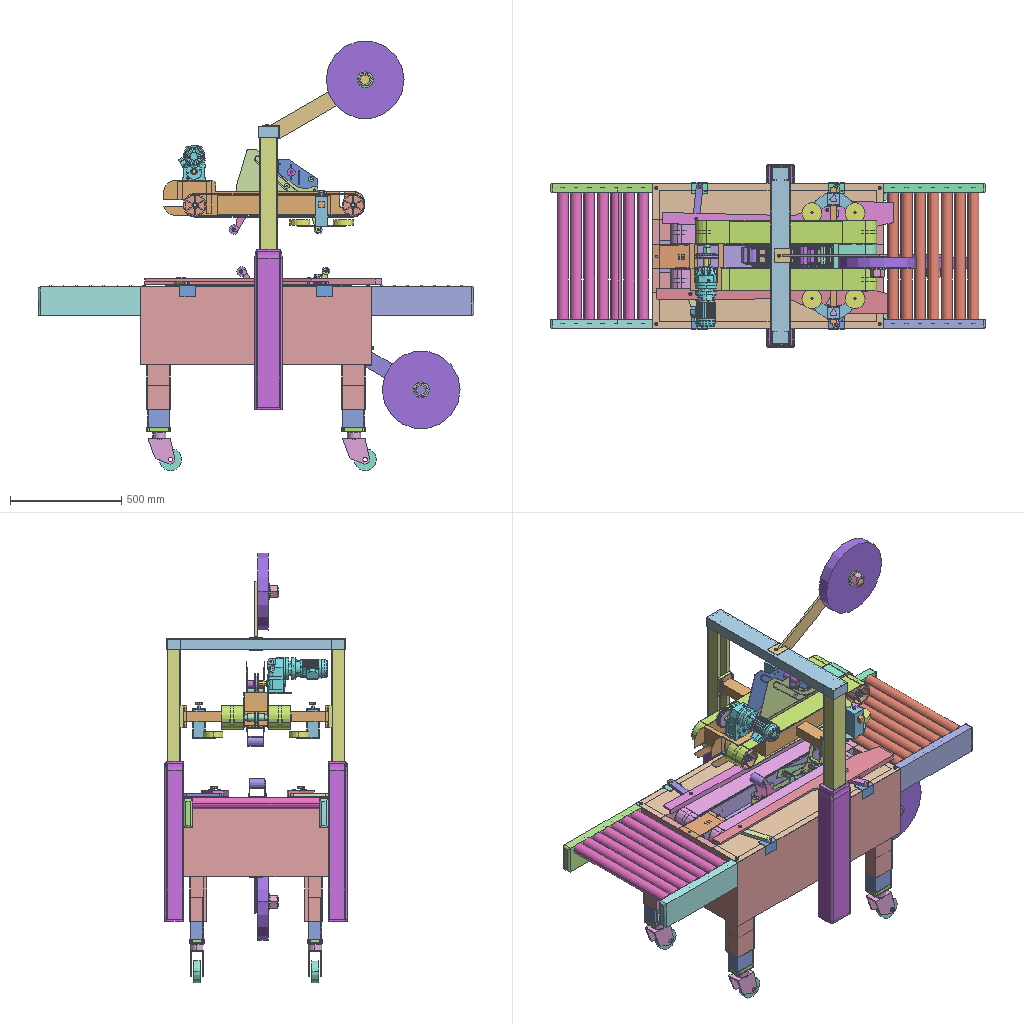Assembly | STEP file | 80 different items | 191 placed | box 1954 x 823 x 1926 mm
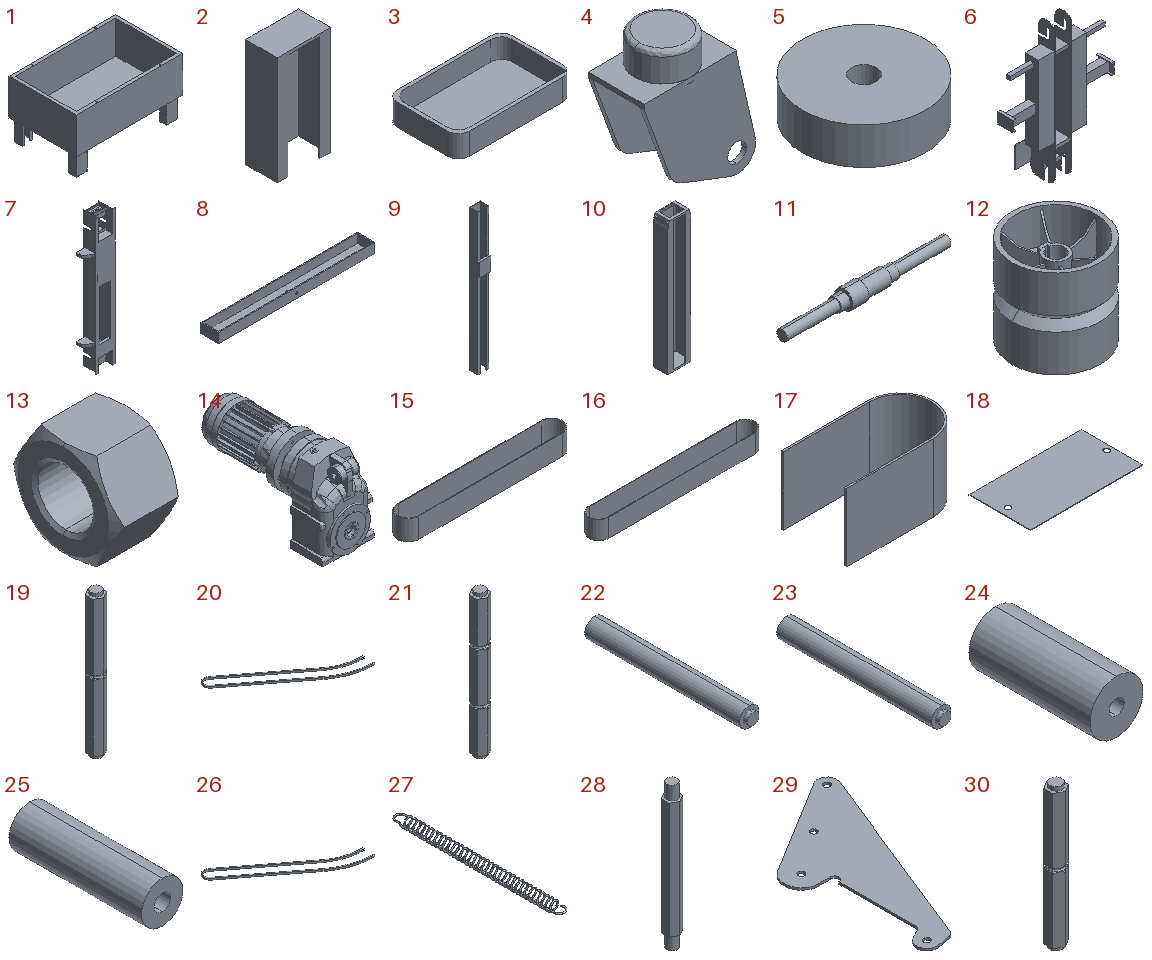Parts list (item | quantity | size | volume):
1 | x1 | 1034 x 650 x 550 mm | 52186602 mm3
2 | x4 | 100 x 60 x 205 mm | 178800 mm3
3 | x4 | 106 x 66 x 20 mm | 31362 mm3
4 | x4 | 120.126 x 60 x 145.273 mm | 22145 mm3
5 | x4 | 100 x 100 x 30 mm | 226195 mm3
6 | x1 | 651 x 157 x 900 mm | 11290183 mm3
7 | x1 | 236 x 103 x 974 mm | 2291572 mm3
8 | x1 | 807 x 90 x 50 mm | 761515 mm3
9 | x2 | 80 x 73 x 1000 mm | 784880 mm3
10 | x2 | 126 x 86 x 720 mm | 848625 mm3
11 | x4 | 310 x 35 x 35 mm | 140893 mm3
12 | x8 | 100 x 100 x 100 mm | 282677 mm3
13 | x4 | 16.4 x 27.713 x 24 mm | 5590 mm3
14 | x2 | 121.404 x 271.25 x 157.01 mm | 2000686 mm3
15 | x2 | 816 x 106 x 100 mm | 523075 mm3
16 | x2 | 906 x 106 x 100 mm | 577075 mm3
17 | x1 | 193 x 106 x 110 mm | 145791 mm3
18 | x1 | 202.5 x 110 x 1 mm | 22118 mm3
19 | x2 | 8 x 9.238 x 84 mm | 4524 mm3
20 | x2 | 261.956 x 181.154 x 4 mm | 7579 mm3
21 | x2 | 8 x 9.238 x 84 mm | 4502 mm3
22 | x2 | 10 x 82 x 10 mm | 6340 mm3
23 | x2 | 10 x 82 x 10 mm | 6340 mm3
24 | x2 | 35 x 80 x 35 mm | 70686 mm3
25 | x2 | 25 x 80 x 25 mm | 32987 mm3
26 | x2 | 261.956 x 181.154 x 4 mm | 7579 mm3
27 | x2 | 9.014 x 139 x 9.007 mm | 726.563 mm3
28 | x2 | 8 x 9.238 x 84 mm | 4221 mm3
29 | x4 | 109 x 190.824 x 2 mm | 17033 mm3
30 | x2 | 8 x 9.238 x 72 mm | 3859 mm3
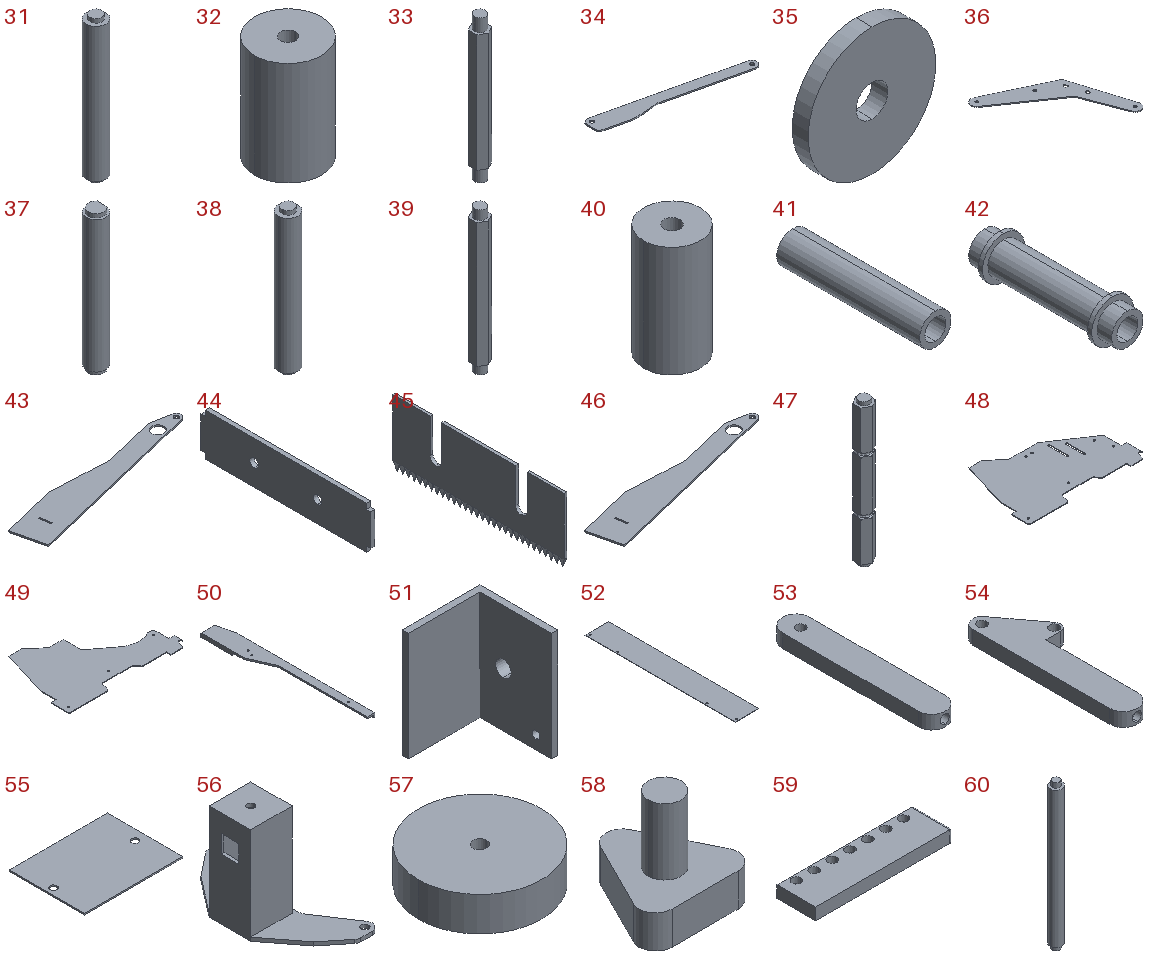31 | x2 | 10 x 10 x 72 mm | 5454 mm3
32 | x2 | 44 x 44 x 68 mm | 98055 mm3
33 | x4 | 8 x 9.238 x 78 mm | 3943 mm3
34 | x4 | 222 x 64 x 2 mm | 8617 mm3
35 | x8 | 24 x 3 x 24 mm | 1272 mm3
36 | x4 | 186 x 204 x 2 mm | 17144 mm3
37 | x4 | 10 x 10 x 72 mm | 5529 mm3
38 | x2 | 10 x 10 x 72 mm | 5454 mm3
39 | x2 | 8 x 9.238 x 78 mm | 4052 mm3
40 | x2 | 35 x 35 x 68 mm | 60083 mm3
41 | x2 | 15 x 68 x 15 mm | 6676 mm3
42 | x2 | 20 x 68 x 20 mm | 7226 mm3
43 | x2 | 242.784 x 71.457 x 2 mm | 14415 mm3
44 | x2 | 2 x 80 x 20 mm | 3110 mm3
45 | x2 | 1 x 60 x 23 mm | 1151 mm3
46 | x2 | 242.784 x 71.457 x 2 mm | 14415 mm3
47 | x2 | 8 x 9.238 x 80 mm | 4280 mm3
48 | x2 | 398.474 x 263.708 x 2 mm | 144459 mm3
49 | x2 | 398.474 x 264.335 x 2 mm | 117575 mm3
50 | x1 | 120 x 1034 x 25 mm | 939315 mm3
51 | x2 | 65 x 50 x 70 mm | 27960 mm3
52 | x2 | 162.5 x 1034 x 2 mm | 335422 mm3
53 | x1 | 30 x 180 x 15 mm | 74584 mm3
54 | x1 | 53 x 175 x 15 mm | 79206 mm3
55 | x1 | 144 x 110 x 2 mm | 31366 mm3
56 | x2 | 102.124 x 213.51 x 135 mm | 177553 mm3
57 | x4 | 90 x 90 x 25 mm | 157080 mm3
58 | x4 | 30 x 30 x 30 mm | 7592 mm3
59 | x1 | 460 x 130 x 40 mm | 2286127 mm3
60 | x7 | 50 x 50 x 610 mm | 1147467 mm3
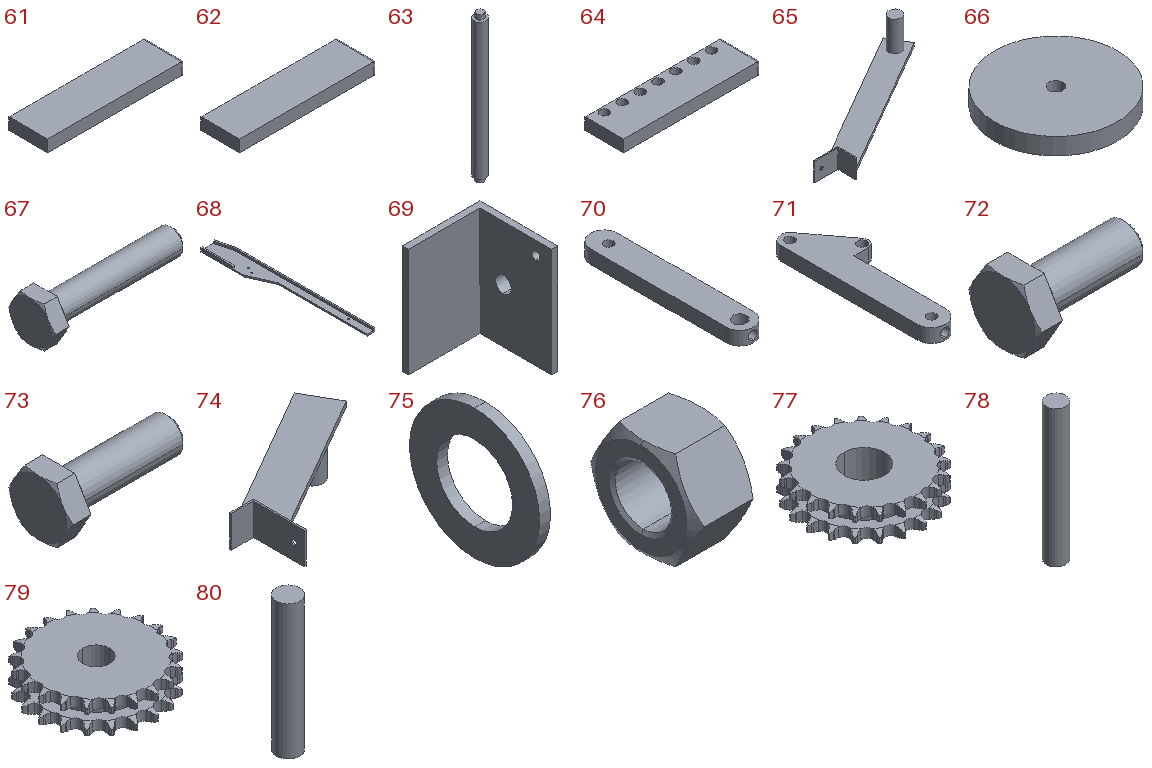61 | x1 | 460 x 130 x 40 mm | 2286127 mm3
62 | x1 | 460 x 130 x 40 mm | 2286127 mm3
63 | x7 | 50 x 50 x 610 mm | 1147467 mm3
64 | x1 | 460 x 130 x 40 mm | 2286127 mm3
65 | x1 | 510.013 x 312.321 x 130 mm | 492742 mm3
66 | x2 | 350 x 350 x 48 mm | 4557823 mm3
67 | x4 | 45.3 x 15.011 x 13 mm | 2753 mm3
68 | x1 | 120 x 1034 x 25 mm | 939315 mm3
69 | x2 | 65 x 50 x 70 mm | 27960 mm3
70 | x1 | 30 x 180 x 15 mm | 74584 mm3
71 | x1 | 53 x 175 x 15 mm | 79206 mm3
72 | x3 | 25.3 x 15.011 x 13 mm | 1750 mm3
73 | x3 | 30.3 x 15.011 x 13 mm | 2001 mm3
74 | x1 | 318.145 x 260.315 x 130 mm | 361674 mm3
75 | x2 | 6 x 72 x 72 mm | 16116 mm3
76 | x2 | 34.7 x 63.509 x 55 mm | 62007 mm3
77 | x2 | 91.67 x 91.415 x 20.973 mm | 80122 mm3
78 | x1 | 20 x 20 x 140 mm | 43982 mm3
79 | x2 | 91.67 x 91.415 x 20.973 mm | 88358 mm3
80 | x1 | 20 x 20 x 115 mm | 36128 mm3
Placements (level | parent | child | x y z in mm | rotation matrix by rows):
1 | subassembly 2 | subassembly 3 | -53.116 -25.809 100.0 | 1 0 0 0 1 0 0 0 1
1 | subassembly 2 | subassembly 4 | 383.884 223.379 -168.0 | -1 0 0 0 1 0 0 0 -1
1 | subassembly 2 | subassembly 5 | 382.389 238.128 -375.0 | 1 0 0 0 1 0 0 0 1
1 | subassembly 2 | subassembly 6 | 386.884 239.191 -405.0 | 1 0 0 0 1 0 0 0 1
1 | subassembly 2 | subassembly 7 | 437.011 239.191 -500.272 | 1 0 0 0 0 -1 0 1 -0
1 | subassembly 2 | subassembly 7 | 437.011 -290.809 -500.272 | 1 0 0 0 0 -1 0 1 0
1 | subassembly 2 | subassembly 5 | 382.389 -291.872 -375.0 | 1 0 0 0 1 0 0 0 1
1 | subassembly 2 | subassembly 6 | 386.884 -290.809 -405.0 | 1 0 0 0 1 0 0 0 1
1 | subassembly 2 | subassembly 4 | 383.884 -274.998 -168.0 | 1 0 0 0 -1 0 0 0 -1
1 | subassembly 2 | subassembly 7 | -436.989 -291.872 -500.272 | 1 0 0 0 0 -1 0 1 -0
1 | subassembly 2 | subassembly 5 | -491.611 -291.872 -375.0 | 1 0 0 0 1 0 0 0 1
1 | subassembly 2 | subassembly 6 | -487.116 -290.809 -405.0 | 1 0 0 0 1 0 0 0 1
1 | subassembly 2 | subassembly 4 | -490.116 -274.998 -168.0 | 1 0 0 0 -1 0 0 0 -1
1 | subassembly 2 | subassembly 7 | -436.989 239.191 -500.272 | 1 0 0 0 0 -1 0 1 -0
1 | subassembly 2 | subassembly 5 | -491.611 238.128 -375.0 | 1 0 0 0 1 0 0 0 1
1 | subassembly 2 | subassembly 6 | -487.116 239.191 -405.0 | 1 0 0 0 1 0 0 0 1
1 | subassembly 2 | subassembly 4 | -490.116 223.379 -168.0 | -1 0 0 0 1 0 0 0 -1
1 | subassembly 2 | subassembly 8 | -467.116 -26.309 674.0 | 0 0 1 1 0 0 0 1 -0
1 | subassembly 2 | subassembly 9 | 459.884 -32.309 250.0 | 0 0 -1 -1 0 0 0 1 0
1 | subassembly 2 | subassembly 10 | -26.761 -240.844 997.0 | 0 -1 0 -1 0 0 0 0 -1
1 | subassembly 2 | subassembly 11 | 4.294 334.08 -8.0 | 1 0 0 0 1 0 0 0 1
1 | subassembly 2 | subassembly 11 | 1.475 -386.699 -8.0 | -1 0 0 0 -1 0 0 0 1
1 | subassembly 2 | subassembly 12 | 30.799 -401.975 -265.0 | -1 0 0 0 -1 0 0 0 1
1 | subassembly 2 | subassembly 12 | -25.03 349.356 -265.0 | 1 0 0 0 1 0 0 0 1
1 | subassembly 2 | subassembly 13 | -438.828 -23.71 230.555 | 0 -0.9184 0.3956 -1 0 0 0 -0.3956 -0.9184
2 | subassembly 13 | subassembly 14 | -183.48 31.868 -0.0 | 1 0 0 0 1 0 0 0 1
3 | subassembly 14 | subassembly 15 | 34.079 -30.465 0.0 | 1 0 0 0 1 0 0 0 1
4 | subassembly 15 | subassembly 16 | -0.0 0.0 -0.0 | 1 0 0 0 1 0 0 0 1
2 | subassembly 13 | subassembly 17 | -101.4 1.402 -0.0 | 0 0 -1 0 1 0 1 0 0
2 | subassembly 13 | subassembly 17 | 112.6 1.402 -0.0 | 0 0 -1 0 1 0 1 0 0
2 | subassembly 13 | subassembly 18 | 164 1.402 -0.0 | -1 0 0 0 -1 0 0 0 1
1 | subassembly 2 | subassembly 13 | 381.482 -20.71 641.0 | 0 1 0 -1 0 0 0 0 1
2 | subassembly 13 | subassembly 14 | -183.48 31.868 -0.0 | 1 0 0 0 1 0 0 0 1
3 | subassembly 14 | subassembly 15 | 34.079 -30.465 0.0 | 1 0 0 0 1 0 0 0 1
4 | subassembly 15 | subassembly 16 | -0.0 0.0 -0.0 | 1 0 0 0 1 0 0 0 1
2 | subassembly 13 | subassembly 17 | -101.4 1.402 -0.0 | 0 0 -1 0 1 0 1 0 0
2 | subassembly 13 | subassembly 17 | 112.6 1.402 -0.0 | 0 0 -1 0 1 0 1 0 0
2 | subassembly 13 | subassembly 18 | 164 1.402 -0.0 | -1 0 0 0 -1 0 0 0 1
1 | subassembly 2 | subassembly 13 | 360.08 -23.71 228.611 | 0 -0.1395 -0.9902 -1 0 0 0 0.9902 -0.1395
2 | subassembly 13 | subassembly 14 | -183.48 31.868 -0.0 | 1 0 0 0 1 0 0 0 1
3 | subassembly 14 | subassembly 15 | 34.079 -30.465 0.0 | 1 0 0 0 1 0 0 0 1
4 | subassembly 15 | subassembly 16 | -0.0 0.0 -0.0 | 1 0 0 0 1 0 0 0 1
2 | subassembly 13 | subassembly 17 | -101.4 1.402 -0.0 | 0 0 -1 0 1 0 1 0 0
2 | subassembly 13 | subassembly 17 | 112.6 1.402 -0.0 | 0 0 -1 0 1 0 1 0 0
2 | subassembly 13 | subassembly 18 | 164 1.402 -0.0 | -1 0 0 0 -1 0 0 0 1
1 | subassembly 2 | subassembly 13 | -328.518 -20.71 641.0 | 0 1 0 -1 0 0 0 0 1
2 | subassembly 13 | subassembly 14 | -183.48 31.868 -0.0 | 1 0 0 0 1 0 0 0 1
3 | subassembly 14 | subassembly 15 | 34.079 -30.465 0.0 | 1 0 0 0 1 0 0 0 1
4 | subassembly 15 | subassembly 16 | -0.0 0.0 -0.0 | 1 0 0 0 1 0 0 0 1
2 | subassembly 13 | subassembly 17 | -101.4 1.402 -0.0 | 0 0 -1 0 1 0 1 0 0
2 | subassembly 13 | subassembly 17 | 112.6 1.402 -0.0 | 0 0 -1 0 1 0 1 0 0
2 | subassembly 13 | subassembly 18 | 164 1.402 -0.0 | -1 0 0 0 -1 0 0 0 1
1 | subassembly 2 | subassembly 19 | -440.116 -98.559 -4.05 | -1 0 0 0 -1 0 0 0 1
1 | subassembly 2 | subassembly 20 | -167.646 -183.309 647.408 | 1 0 0 0 0 1 0 -1 0
1 | subassembly 2 | subassembly 20 | -167.646 30.691 647.408 | 1 0 0 0 0 1 0 -1 0
1 | subassembly 2 | subassembly 21 | -280.646 -86.309 223.593 | 1 0 0 0 0 -1 0 1 0
1 | subassembly 2 | subassembly 21 | -280.646 127.691 223.593 | 1 0 0 0 0 -1 0 1 0
1 | subassembly 2 | subassembly 22 | 355.25 -81.309 627.099 | 1 0 0 0 0 1 0 -1 0
1 | subassembly 2 | subassembly 23 | -516.823 -37.75 276.0 | 1 0 0 0 -1 0 0 0 -1
1 | subassembly 2 | subassembly 24 | -139.589 15.691 645.0 | 1 0 0 0 0 -1 0 1 0
2 | subassembly 24 | subassembly 25 | 173.458 14.311 21.465 | 0.9755 -0.2201 0 -0.2201 -0.9755 0 0 0 -1
2 | subassembly 24 | subassembly 26 | 170.281 106.032 -0.0 | 0.9943 0.1069 0 -0.1069 0.9943 0 0 0 1
2 | subassembly 24 | subassembly 27 | 357.869 44.999 21.465 | 1 0 0 0 -1 0 0 0 -1
2 | subassembly 24 | subassembly 28 | 244.449 145.206 -2.0 | -0.03127 0 -0.9995 -0.9995 0 0.03127 0 1 -0
2 | subassembly 24 | subassembly 29 | 334.449 115.101 -2.0 | 1 0 0 0 0 -1 0 1 -0
2 | subassembly 24 | subassembly 30 | 244.449 145.206 -0.0 | 1 0 0 0 0 -1 0 1 0
2 | subassembly 24 | subassembly 31 | 334.449 115.101 0.0 | 1 0 0 0 0 -1 0 1 0
2 | subassembly 24 | subassembly 32 | 170.281 106.032 80.0 | 0.9943 0.1069 0 -0.1069 0.9943 0 0 0 1
2 | subassembly 24 | subassembly 33 | 166.405 36.035 40.0 | 0.05894 -0.9983 0 -0.9983 -0.05894 0 0 0 -1
3 | subassembly 33 | subassembly 34 | -0.0 -0.0 -0.0 | 1 0 0 0 1 0 0 0 1
2 | subassembly 24 | subassembly 35 | 8.419 20.574 58.535 | 1 0 0 0 1 0 0 0 1
2 | subassembly 24 | subassembly 36 | -0.0 -0.0 -0.0 | 0.9885 0.1511 0 -0.1511 0.9885 0 0 0 1
3 | subassembly 36 | subassembly 37 | 172.931 87.653 4.0 | 1 0 0 0 1 0 0 0 1
3 | subassembly 36 | subassembly 38 | 58.007 15.537 58.535 | -0.2359 0.9718 0 -0.9718 -0.2359 0 0 0 1
3 | subassembly 36 | subassembly 37 | 172.931 87.653 74.0 | 1 0 0 0 1 0 0 0 1
3 | subassembly 36 | subassembly 39 | -194.099 -291.8 40.0 | 0.9934 -0.1146 0 -0.1146 -0.9934 0 0 0 -1
3 | subassembly 36 | subassembly 40 | -260.32 -109.992 40.0 | -0.6453 -0.764 0 0.764 -0.6453 0 0 0 1
2 | subassembly 24 | subassembly 41 | 25.745 -32.456 -0.0 | 0.996 -0.08979 0 0.08979 0.996 0 0 0 1
3 | subassembly 41 | subassembly 42 | 91.173 59.732 58.535 | -0.2375 0.9714 0 -0.9714 -0.2375 0 0 0 1
3 | subassembly 41 | subassembly 42 | 300.733 27.296 58.535 | -0.1825 0.9832 0 -0.9832 -0.1825 0 0 0 1
3 | subassembly 41 | subassembly 43 | 159.966 106.605 4.0 | 0.9975 -0.06997 0 0.06997 0.9975 0 0 0 1
3 | subassembly 41 | subassembly 43 | 159.966 106.605 70.0 | 0.9975 -0.06997 0 0.06997 0.9975 0 0 0 1
2 | subassembly 24 | subassembly 44 | 21.019 -28.999 -0.0 | 0.9966 -0.0823 0 0.0823 0.9966 0 0 0 1
3 | subassembly 44 | subassembly 45 | 286.164 37.612 1.0 | -0.7245 0 0.6893 0.6893 0 0.7245 0 1 -0
3 | subassembly 44 | subassembly 45 | 211.519 94.196 4.0 | 0.3873 0 0.922 -0.922 0 0.3873 0 -1 -0
3 | subassembly 44 | subassembly 46 | 183.108 121.677 4.0 | 0.9822 0.1879 0 -0.1879 0.9822 0 0 0 1
3 | subassembly 44 | subassembly 47 | 298.935 -14.379 6.0 | 0.9398 -0.3416 0 0.3416 0.9398 0 0 0 1
3 | subassembly 44 | subassembly 47 | 297.053 -36.9 6.0 | 0.9822 0.1879 0 -0.1879 0.9822 0 0 0 1
3 | subassembly 44 | subassembly 48 | 184.87 107.772 40.0 | 0.9929 0.119 0 -0.119 0.9929 0 0 0 1
3 | subassembly 44 | subassembly 46 | 183.108 121.677 74.0 | 0.9822 0.1879 0 -0.1879 0.9822 0 0 0 1
3 | subassembly 44 | subassembly 45 | 211.519 94.196 79.0 | 0.719 0 -0.695 0.695 0 0.719 0 -1 0
3 | subassembly 44 | subassembly 45 | 286.164 37.612 79.0 | 0.717 0 -0.697 0.697 0 0.717 0 -1 0
3 | subassembly 44 | subassembly 49 | 219.938 73.622 21.465 | 1 0 0 0 -1 0 0 0 -1
3 | subassembly 44 | subassembly 50 | 149.285 -304.553 40.0 | -0.07391 -0.9973 0 0.9973 -0.07391 0 0 0 1
3 | subassembly 44 | subassembly 51 | 327.894 -31.918 6.0 | -0.8023 0 -0.5969 -0.5969 0 0.8023 0 1 0
3 | subassembly 44 | subassembly 52 | 322.872 5.696 74.0 | 0.9831 0 0.1828 -0.1828 0 0.9831 0 -1 -0
2 | subassembly 24 | subassembly 53 | 8.775 -77.882 -0.0 | 0.9749 -0.2225 0 0.2225 0.9749 0 0 0 1
3 | subassembly 53 | subassembly 54 | 189 110.408 -0.0 | 0.9851 0.1717 0 -0.1717 0.9851 0 0 0 1
3 | subassembly 53 | subassembly 55 | 171.282 1.538 40.0 | 1 0 0.006478 -0.006478 0 1 0 -1 -0
3 | subassembly 53 | subassembly 56 | 173.251 -3.373 40.0 | 1 0 0.006478 -0.006478 0 1 0 -1 -0
3 | subassembly 53 | subassembly 57 | 189 110.408 80.0 | 0.9851 0.1717 0 -0.1717 0.9851 0 0 0 1
3 | subassembly 53 | subassembly 58 | 397.672 4.202 21.465 | 0.09404 0.9956 0 0.9956 -0.09404 0 0 0 -1
2 | subassembly 24 | subassembly 59 | -0.0 -0.0 -0.0 | 1 0 0 0 1 0 0 0 1
3 | subassembly 59 | subassembly 60 | -0.0 -0.0 -0.0 | 1 0 0 0 1 0 0 0 1
3 | subassembly 59 | subassembly 61 | -0.0 0.0 82.0 | 1 0 0 0 1 0 0 0 1
1 | subassembly 2 | subassembly 24 | -105.116 -71.309 231.896 | 1 0 0 0 0 1 0 -1 0
2 | subassembly 24 | subassembly 25 | 173.458 14.311 21.465 | 0.9755 -0.2201 0 -0.2201 -0.9755 0 0 0 -1
2 | subassembly 24 | subassembly 26 | 170.281 106.032 -0.0 | 0.9943 0.1069 0 -0.1069 0.9943 0 0 0 1
2 | subassembly 24 | subassembly 27 | 357.869 44.999 21.465 | 1 0 0 0 -1 0 0 0 -1
2 | subassembly 24 | subassembly 28 | 244.449 145.206 -2.0 | -0.03127 0 -0.9995 -0.9995 0 0.03127 0 1 -0
2 | subassembly 24 | subassembly 29 | 334.449 115.101 -2.0 | 1 0 0 0 0 -1 0 1 -0
2 | subassembly 24 | subassembly 30 | 244.449 145.206 -0.0 | 1 0 0 0 0 -1 0 1 0
2 | subassembly 24 | subassembly 31 | 334.449 115.101 0.0 | 1 0 0 0 0 -1 0 1 0
2 | subassembly 24 | subassembly 32 | 170.281 106.032 80.0 | 0.9943 0.1069 0 -0.1069 0.9943 0 0 0 1
2 | subassembly 24 | subassembly 33 | 166.405 36.035 40.0 | 0.05894 -0.9983 0 -0.9983 -0.05894 0 0 0 -1
3 | subassembly 33 | subassembly 34 | -0.0 -0.0 -0.0 | 1 0 0 0 1 0 0 0 1
2 | subassembly 24 | subassembly 35 | 8.419 20.574 58.535 | 1 0 0 0 1 0 0 0 1
2 | subassembly 24 | subassembly 36 | -0.0 -0.0 -0.0 | 0.9885 0.1511 0 -0.1511 0.9885 0 0 0 1
3 | subassembly 36 | subassembly 37 | 172.931 87.653 4.0 | 1 0 0 0 1 0 0 0 1
3 | subassembly 36 | subassembly 38 | 58.007 15.537 58.535 | -0.2359 0.9718 0 -0.9718 -0.2359 0 0 0 1
3 | subassembly 36 | subassembly 37 | 172.931 87.653 74.0 | 1 0 0 0 1 0 0 0 1
3 | subassembly 36 | subassembly 39 | -194.099 -291.8 40.0 | 0.9934 -0.1146 0 -0.1146 -0.9934 0 0 0 -1
3 | subassembly 36 | subassembly 40 | -260.32 -109.992 40.0 | -0.6453 -0.764 0 0.764 -0.6453 0 0 0 1
2 | subassembly 24 | subassembly 41 | 25.745 -32.456 -0.0 | 0.996 -0.08979 0 0.08979 0.996 0 0 0 1
3 | subassembly 41 | subassembly 42 | 91.173 59.732 58.535 | -0.2375 0.9714 0 -0.9714 -0.2375 0 0 0 1
3 | subassembly 41 | subassembly 42 | 300.733 27.296 58.535 | -0.1825 0.9832 0 -0.9832 -0.1825 0 0 0 1
3 | subassembly 41 | subassembly 43 | 159.966 106.605 4.0 | 0.9975 -0.06997 0 0.06997 0.9975 0 0 0 1
3 | subassembly 41 | subassembly 43 | 159.966 106.605 70.0 | 0.9975 -0.06997 0 0.06997 0.9975 0 0 0 1
2 | subassembly 24 | subassembly 44 | 21.019 -28.999 -0.0 | 0.9966 -0.0823 0 0.0823 0.9966 0 0 0 1
3 | subassembly 44 | subassembly 45 | 286.164 37.612 1.0 | -0.7245 0 0.6893 0.6893 0 0.7245 0 1 -0
3 | subassembly 44 | subassembly 45 | 211.519 94.196 4.0 | 0.3873 0 0.922 -0.922 0 0.3873 0 -1 -0
3 | subassembly 44 | subassembly 46 | 183.108 121.677 4.0 | 0.9822 0.1879 0 -0.1879 0.9822 0 0 0 1
3 | subassembly 44 | subassembly 47 | 298.935 -14.379 6.0 | 0.9398 -0.3416 0 0.3416 0.9398 0 0 0 1
3 | subassembly 44 | subassembly 47 | 297.053 -36.9 6.0 | 0.9822 0.1879 0 -0.1879 0.9822 0 0 0 1
3 | subassembly 44 | subassembly 48 | 184.87 107.772 40.0 | 0.9929 0.119 0 -0.119 0.9929 0 0 0 1
3 | subassembly 44 | subassembly 46 | 183.108 121.677 74.0 | 0.9822 0.1879 0 -0.1879 0.9822 0 0 0 1
3 | subassembly 44 | subassembly 45 | 211.519 94.196 79.0 | 0.719 0 -0.695 0.695 0 0.719 0 -1 0
3 | subassembly 44 | subassembly 45 | 286.164 37.612 79.0 | 0.717 0 -0.697 0.697 0 0.717 0 -1 0
3 | subassembly 44 | subassembly 49 | 219.938 73.622 21.465 | 1 0 0 0 -1 0 0 0 -1
3 | subassembly 44 | subassembly 50 | 149.285 -304.553 40.0 | -0.07391 -0.9973 0 0.9973 -0.07391 0 0 0 1
3 | subassembly 44 | subassembly 51 | 327.894 -31.918 6.0 | -0.8023 0 -0.5969 -0.5969 0 0.8023 0 1 0
3 | subassembly 44 | subassembly 52 | 322.872 5.696 74.0 | 0.9831 0 0.1828 -0.1828 0 0.9831 0 -1 -0
2 | subassembly 24 | subassembly 53 | 8.775 -77.882 -0.0 | 0.9749 -0.2225 0 0.2225 0.9749 0 0 0 1
3 | subassembly 53 | subassembly 54 | 189 110.408 -0.0 | 0.9851 0.1717 0 -0.1717 0.9851 0 0 0 1
3 | subassembly 53 | subassembly 55 | 171.282 1.538 40.0 | 1 0 0.006478 -0.006478 0 1 0 -1 -0
3 | subassembly 53 | subassembly 56 | 173.251 -3.373 40.0 | 1 0 0.006478 -0.006478 0 1 0 -1 -0
3 | subassembly 53 | subassembly 57 | 189 110.408 80.0 | 0.9851 0.1717 0 -0.1717 0.9851 0 0 0 1
3 | subassembly 53 | subassembly 58 | 397.672 4.202 21.465 | 0.09404 0.9956 0 0.9956 -0.09404 0 0 0 -1
2 | subassembly 24 | subassembly 59 | -0.0 -0.0 -0.0 | 1 0 0 0 1 0 0 0 1
3 | subassembly 59 | subassembly 60 | -0.0 -0.0 -0.0 | 1 0 0 0 1 0 0 0 1
3 | subassembly 59 | subassembly 61 | -0.0 0.0 82.0 | 1 0 0 0 1 0 0 0 1
1 | subassembly 2 | subassembly 62 | -98.831 137.32 301.0 | -0.02433 0.9997 0 -0.9997 -0.02433 0 0 0 1
1 | subassembly 2 | subassembly 63 | -325.116 283.789 246.897 | 0 0 -1 0 1 0 1 0 -0
1 | subassembly 2 | subassembly 63 | 288.884 283.789 246.897 | 0 0 -1 0 1 0 1 0 0
1 | subassembly 2 | subassembly 64 | -468.567 -280.079 275.0 | 0 -1 0 1 0 0 0 0 1
1 | subassembly 2 | subassembly 64 | -468.567 228.461 277.0 | 0 -1 0 -1 0 0 0 0 -1
1 | subassembly 2 | subassembly 65 | -379.508 139.677 286.0 | -0.9943 -0.1069 0 0.1069 -0.9943 0 0 0 1
1 | subassembly 2 | subassembly 66 | 196.576 205.656 301.0 | -0.9952 -0.09753 0 0.09753 -0.9952 0 0 0 1
1 | subassembly 2 | subassembly 67 | 411.966 -62.962 275.0 | 1 0 0 0 1 0 0 0 1
1 | subassembly 2 | subassembly 68 | 240.976 229.691 546.5 | 0 1 0 -1 0 0 0 0 1
1 | subassembly 2 | subassembly 68 | 240.976 -282.309 546.5 | 0 -1 0 1 0 0 0 0 1
1 | subassembly 2 | subassembly 69 | 337.731 166.567 576.5 | 1 0 0 0 -1 0 0 0 -1
1 | subassembly 2 | subassembly 69 | 144.221 166.567 576.5 | 1 0 0 0 -1 0 0 0 -1
1 | subassembly 2 | subassembly 69 | 144.221 -219.185 576.5 | 1 0 0 0 -1 0 0 0 -1
1 | subassembly 2 | subassembly 69 | 337.731 -219.185 576.5 | 1 0 0 0 -1 0 0 0 -1
1 | subassembly 2 | subassembly 70 | 243.778 -254.689 706.5 | -0.9949 0.1009 0 0.1009 0.9949 0 0 0 -1
1 | subassembly 2 | subassembly 70 | 248.181 256.501 706.5 | -0.9657 0.2595 0 0.2595 0.9657 0 0 0 -1
1 | subassembly 2 | subassembly 71 | 693.884 299.191 212.0 | 1 0 0 0 0 -1 0 1 0
1 | subassembly 2 | subassembly 72 | 808.884 -310.809 257.0 | 1 0 0 0 0 1 0 -1 0
1 | subassembly 2 | subassembly 72 | 568.884 -310.809 257.0 | 1 0 0 0 0 1 0 -1 0
1 | subassembly 2 | subassembly 72 | 508.884 -310.809 257.0 | 1 0 0 0 0 1 0 -1 0
1 | subassembly 2 | subassembly 72 | 628.884 -310.809 257.0 | 1 0 0 0 0 1 0 -1 0
1 | subassembly 2 | subassembly 72 | 688.884 -310.809 257.0 | 1 0 0 0 0 1 0 -1 0
1 | subassembly 2 | subassembly 72 | 748.884 -310.809 257.0 | 1 0 0 0 0 1 0 -1 0
1 | subassembly 2 | subassembly 72 | 868.884 -310.809 257.0 | 1 0 0 0 0 1 0 -1 0
1 | subassembly 2 | subassembly 73 | 693.884 -350.809 212.0 | 1 0 0 0 0 -1 0 1 -0
1 | subassembly 2 | subassembly 74 | -800.116 299.191 210.0 | -1 0 0 0 0 1 0 1 0
1 | subassembly 2 | subassembly 75 | -915.116 -310.809 255.0 | -0.9831 0.1832 0 0 0 -1 -0.1832 -0.9831 -0
1 | subassembly 2 | subassembly 75 | -675.116 -310.809 255.0 | -0.9747 0.2235 0 0 0 -1 -0.2235 -0.9747 -0
1 | subassembly 2 | subassembly 75 | -615.116 -310.809 255.0 | -1 0.004816 0 0 0 -1 -0.004816 -1 -0
1 | subassembly 2 | subassembly 75 | -735.116 -310.809 255.0 | -0.4278 0.9039 0 0 0 -1 -0.9039 -0.4278 -0
1 | subassembly 2 | subassembly 75 | -795.116 -310.809 255.0 | -0.9979 0.06501 0 0 0 -1 -0.06501 -0.9979 -0
1 | subassembly 2 | subassembly 75 | -855.116 -310.809 255.0 | -0.9955 0.09517 0 0 0 -1 -0.09517 -0.9955 -0
1 | subassembly 2 | subassembly 75 | -975.116 -310.809 255.0 | -0.9999 -0.01077 0 0 0 -1 0.01077 -0.9999 -0
1 | subassembly 2 | subassembly 76 | -800.116 -350.809 210.0 | -1 0 0 0 0 1 0 1 0
1 | subassembly 2 | subassembly 77 | -0.371 -26.309 970.39 | 1 0 0 0 0 -1 0 1 -0
1 | subassembly 2 | subassembly 78 | 436.726 -82.309 1204.363 | 1 0 0 0 0 1 0 -1 0
1 | subassembly 2 | subassembly 79 | 448.884 -330.809 277.0 | 0 -1 0 0 0 1 -1 0 -0
1 | subassembly 2 | subassembly 79 | 448.884 279.191 277.0 | 0 -1 0 0 0 1 -1 0 0
1 | subassembly 2 | subassembly 79 | -555.116 -330.809 277.0 | 0 -1 0 0 0 1 -1 0 -0
1 | subassembly 2 | subassembly 79 | -555.116 279.191 277.0 | 0 -1 0 0 0 1 -1 0 0
1 | subassembly 2 | subassembly 70 | 226.85 -203.534 331.0 | -0.9992 0.03882 0 0.03882 0.9992 0 0 0 -1
1 | subassembly 2 | subassembly 70 | 224.518 165.93 331.0 | -0.0783 -0.9969 0 -0.9969 0.0783 0 0 0 -1
1 | subassembly 2 | subassembly 80 | -124.752 -198.866 301.0 | -0.007303 1 0 1 0.007303 0 0 0 -1
1 | subassembly 2 | subassembly 81 | -325.116 -335.408 246.897 | 0 0 1 0 -1 0 1 0 0
1 | subassembly 2 | subassembly 81 | 288.884 -335.408 246.897 | 0 0 1 0 -1 0 1 0 0
1 | subassembly 2 | subassembly 82 | -405.434 -197.222 286.0 | -0.9583 -0.2857 0 -0.2857 0.9583 0 0 0 -1
1 | subassembly 2 | subassembly 83 | 177.294 -275.927 301.0 | -0.9307 -0.3658 0 -0.3658 0.9307 0 0 0 -1
1 | subassembly 2 | subassembly 84 | -375.621 140.022 311.0 | 0 -0.9999 0.01703 0 0.01703 0.9999 -1 0 0
1 | subassembly 2 | subassembly 85 | -401.549 -196.855 311.0 | 0 -1 0 0 0 1 -1 0 -0
1 | subassembly 2 | subassembly 85 | 185.89 -247.566 311.0 | 0 -1 0 0 0 1 -1 0 -0
1 | subassembly 2 | subassembly 85 | 212.596 180.724 311.0 | 0 -0.9999 0.01703 0 0.01703 0.9999 -1 0 0
1 | subassembly 2 | subassembly 86 | 415.629 -25.809 -48.39 | 1 0 0 0 0 1 0 -1 0
1 | subassembly 2 | subassembly 84 | -4.116 -26.309 1000.0 | 0 -1 0 0 0 1 -1 0 0
1 | subassembly 2 | subassembly 84 | 466.884 -25.809 2.0 | -1 0 0 0 -1 0 0 0 1
1 | subassembly 2 | subassembly 19 | -331.375 -123.459 792.95 | -1 0 0 0 -1 0 0 0 1
1 | subassembly 2 | subassembly 78 | 688.362 -81.809 -187.417 | 1 0 0 0 0 1 0 -1 0
1 | subassembly 2 | subassembly 87 | 436.726 -82.309 1204.363 | 0 1 0 -1 0 0 0 0 1
1 | subassembly 2 | subassembly 87 | 688.362 -81.809 -187.417 | 0 1 0 -1 0 0 0 0 1
1 | subassembly 2 | subassembly 88 | 436.726 -123.009 1204.363 | 0 -1 0 1 0 0 0 0 1
1 | subassembly 2 | subassembly 88 | 688.362 -122.509 -187.417 | 0 -1 0 1 0 0 0 0 1
1 | subassembly 2 | subassembly 89 | -327.116 -35.756 641.0 | 1 0 0 0 0 1 0 -1 0
1 | subassembly 2 | subassembly 90 | -331.375 -17.059 791.457 | 1 0 0 0 0 -1 0 1 0
1 | subassembly 2 | subassembly 91 | -331.375 -21.836 792.95 | 1 0 0 0 0 -1 0 1 -0
1 | subassembly 2 | subassembly 89 | -440.116 -38.756 230.0 | 1 0 0 0 0 1 0 -1 -0
1 | subassembly 2 | subassembly 91 | -440.116 -24.836 -4.05 | 1 0 0 0 0 -1 0 1 0
1 | subassembly 2 | subassembly 92 | -440.116 -22.159 -5.543 | 1 0 0 0 0 -1 0 1 0